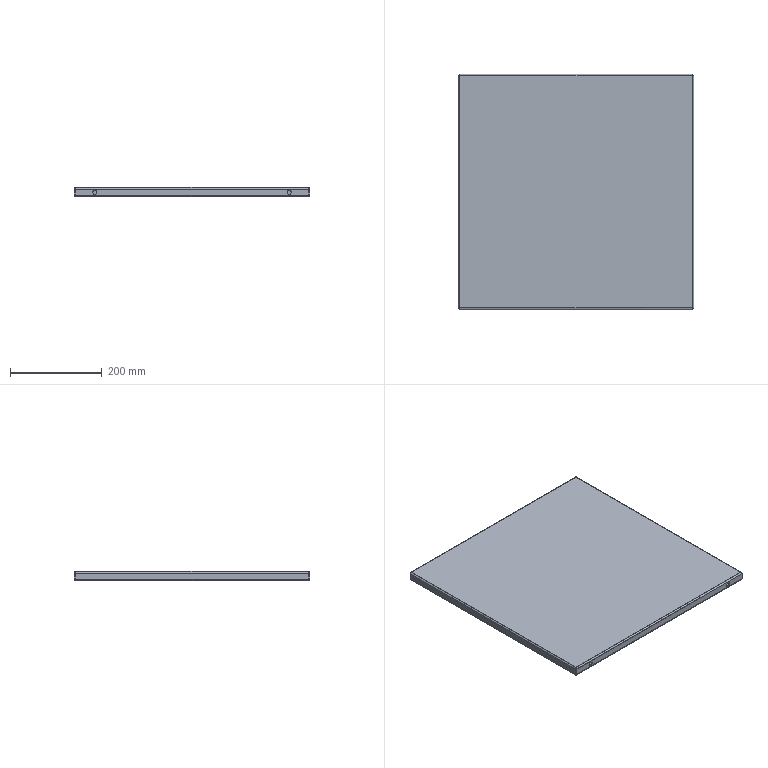Part | STEP file | 750038521 | 1 solid | 66 faces | box 514 x 514 x 20 mm | volume 656019 mm3 | plane 46 | cylinder 20 | commonest cylinder face diameters 2 x4 4 x4 6 x4 8 x4 9 x4